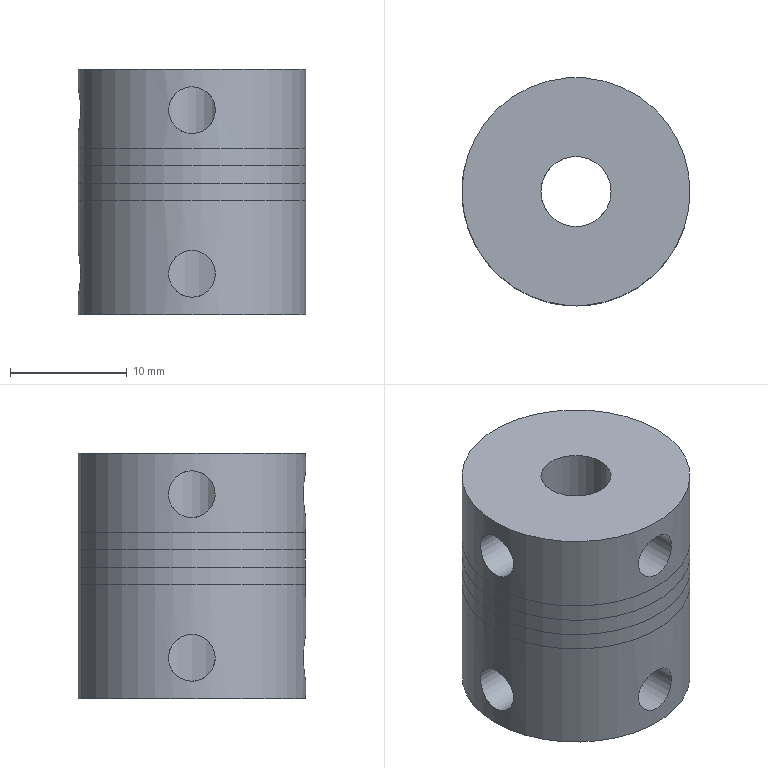Part | STEP file | lianzhouqi | 1 solid | 14 faces | box 19.5 x 19.5 x 21 mm | volume 4222 mm3 | cylinder 11 | plane 3 | commonest cylinder face diameters 19.5 x5 4 x4 6 x1 12 x1